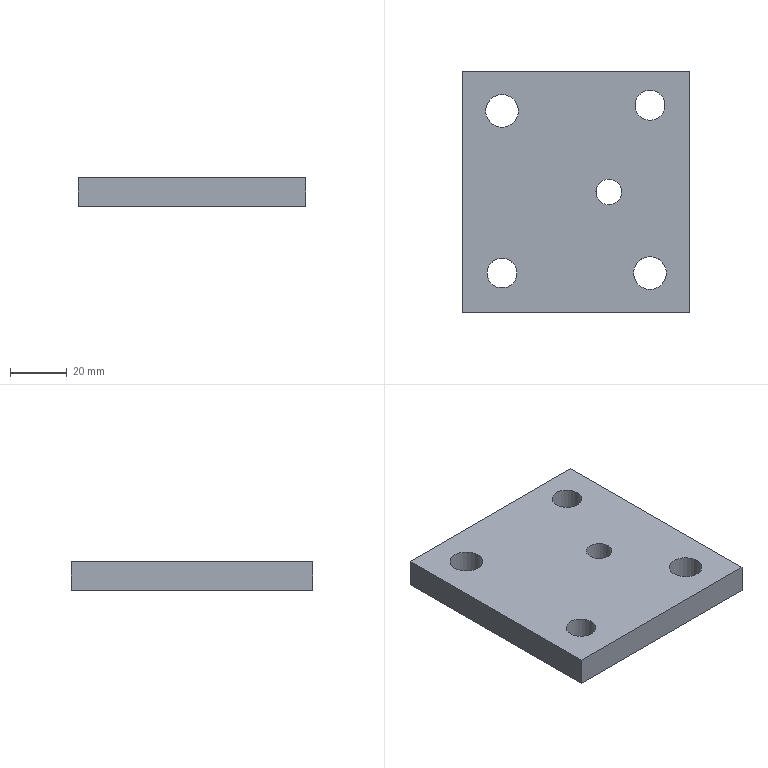Part | NX | features 6 2 | 1 solid | 11 faces | box 80 x 85 x 10 mm | volume 63555 mm3 | plane 6 | cylinder 5 | commonest cylinder face diameters 10.5 x2 11.5 x2 9 x1
STEP:
#1=CARTESIAN_POINT('',(3152.247,119.828,101.));
#2=VERTEX_POINT('',#1);
#3=CARTESIAN_POINT('',(3152.247,34.828,101.));
#4=VERTEX_POINT('',#3);
#5=CARTESIAN_POINT('',(3152.247,77.328,101.));
#6=DIRECTION('',(0.,-1.,0.));
#7=VECTOR('',#6,1000.);
#8=LINE('',#5,#7);
#9=EDGE_CURVE('',#2,#4,#8,.T.);
#10=ORIENTED_EDGE('',*,*,#9,.T.);
#11=CARTESIAN_POINT('',(3152.247,34.828,91.));
#12=VERTEX_POINT('',#11);
#13=CARTESIAN_POINT('',(3152.247,34.828,81.));
#14=DIRECTION('',(0.,0.,1.));
#15=VECTOR('',#14,1000.);
#16=LINE('',#13,#15);
#17=EDGE_CURVE('',#12,#4,#16,.T.);
#18=ORIENTED_EDGE('',*,*,#17,.F.);
#19=CARTESIAN_POINT('',(3152.247,119.828,91.));
#20=VERTEX_POINT('',#19);
#21=CARTESIAN_POINT('',(3152.247,77.328,91.));
#22=DIRECTION('',(0.,-1.,0.));
#23=VECTOR('',#22,1000.);
#24=LINE('',#21,#23);
#25=EDGE_CURVE('',#20,#12,#24,.T.);
#26=ORIENTED_EDGE('',*,*,#25,.F.);
#27=CARTESIAN_POINT('',(3152.247,119.828,81.));
#28=DIRECTION('',(0.,0.,-1.));
#29=VECTOR('',#28,1000.);
#30=LINE('',#27,#29);
#31=EDGE_CURVE('',#2,#20,#30,.T.);
#32=ORIENTED_EDGE('',*,*,#31,.F.);
#33=EDGE_LOOP('',(#10,#18,#26,#32));
#34=FACE_BOUND('',#33,.T.);
#35=CARTESIAN_POINT('',(3152.247,77.328,81.));
#36=DIRECTION('',(-1.,0.,0.));
#37=DIRECTION('',(0.,-1.,0.));
#38=AXIS2_PLACEMENT_3D('',#35,#36,#37);
#39=PLANE('',#38);
#40=ADVANCED_FACE('',(#34),#39,.F.);
#41=CARTESIAN_POINT('',(3072.247,119.828,101.));
#42=VERTEX_POINT('',#41);
#43=CARTESIAN_POINT('',(3102.247,119.828,101.));
#44=DIRECTION('',(1.,0.,0.));
#45=VECTOR('',#44,1000.);
#46=LINE('',#43,#45);
#47=EDGE_CURVE('',#42,#2,#46,.T.);
#48=ORIENTED_EDGE('',*,*,#47,.T.);
#49=ORIENTED_EDGE('',*,*,#31,.T.);
#50=CARTESIAN_POINT('',(3072.247,119.828,91.));
#51=VERTEX_POINT('',#50);
#52=CARTESIAN_POINT('',(3102.247,119.828,91.));
#53=DIRECTION('',(1.,0.,0.));
#54=VECTOR('',#53,1000.);
#55=LINE('',#52,#54);
#56=EDGE_CURVE('',#51,#20,#55,.T.);
#57=ORIENTED_EDGE('',*,*,#56,.F.);
#58=CARTESIAN_POINT('',(3072.247,119.828,81.));
#59=DIRECTION('',(0.,0.,-1.));
#60=VECTOR('',#59,1000.);
#61=LINE('',#58,#60);
#62=EDGE_CURVE('',#42,#51,#61,.T.);
#63=ORIENTED_EDGE('',*,*,#62,.F.);
#64=EDGE_LOOP('',(#48,#49,#57,#63));
#65=FACE_BOUND('',#64,.T.);
#66=CARTESIAN_POINT('',(3102.247,119.828,81.));
#67=DIRECTION('',(0.,-1.,0.));
#68=DIRECTION('',(1.,0.,0.));
#69=AXIS2_PLACEMENT_3D('',#66,#67,#68);
#70=PLANE('',#69);
#71=ADVANCED_FACE('',(#65),#70,.F.);
#72=CARTESIAN_POINT('',(3072.247,34.828,101.));
#73=VERTEX_POINT('',#72);
#74=CARTESIAN_POINT('',(3072.247,77.328,101.));
#75=DIRECTION('',(0.,1.,0.));
#76=VECTOR('',#75,1000.);
#77=LINE('',#74,#76);
#78=EDGE_CURVE('',#73,#42,#77,.T.);
#79=ORIENTED_EDGE('',*,*,#78,.T.);
#80=ORIENTED_EDGE('',*,*,#62,.T.);
#81=CARTESIAN_POINT('',(3072.247,34.828,91.));
#82=VERTEX_POINT('',#81);
#83=CARTESIAN_POINT('',(3072.247,77.328,91.));
#84=DIRECTION('',(0.,1.,0.));
#85=VECTOR('',#84,1000.);
#86=LINE('',#83,#85);
#87=EDGE_CURVE('',#82,#51,#86,.T.);
#88=ORIENTED_EDGE('',*,*,#87,.F.);
#89=CARTESIAN_POINT('',(3072.247,34.828,81.));
#90=DIRECTION('',(0.,0.,-1.));
#91=VECTOR('',#90,1000.);
#92=LINE('',#89,#91);
#93=EDGE_CURVE('',#73,#82,#92,.T.);
#94=ORIENTED_EDGE('',*,*,#93,.F.);
#95=EDGE_LOOP('',(#79,#80,#88,#94));
#96=FACE_BOUND('',#95,.T.);
#97=CARTESIAN_POINT('',(3072.247,77.328,81.));
#98=DIRECTION('',(1.,0.,0.));
#99=DIRECTION('',(0.,1.,0.));
#100=AXIS2_PLACEMENT_3D('',#97,#98,#99);
#101=PLANE('',#100);
#102=ADVANCED_FACE('',(#96),#101,.F.);
#103=CARTESIAN_POINT('',(3091.497,48.828,91.));
#104=VERTEX_POINT('',#103);
#105=CARTESIAN_POINT('',(3086.247,48.828,91.));
#106=DIRECTION('',(0.,0.,-1.));
#107=DIRECTION('',(1.,0.,0.));
#108=AXIS2_PLACEMENT_3D('',#105,#106,#107);
#109=CIRCLE('',#108,5.25);
#110=EDGE_CURVE('',#104,#104,#109,.T.);
#111=ORIENTED_EDGE('',*,*,#110,.T.);
#112=EDGE_LOOP('',(#111));
#113=FACE_BOUND('',#112,.T.);
#114=CARTESIAN_POINT('',(3080.997,48.828,101.));
#115=VERTEX_POINT('',#114);
#116=CARTESIAN_POINT('',(3086.247,48.828,101.));
#117=DIRECTION('',(0.,0.,1.));
#118=DIRECTION('',(-1.,0.,0.));
#119=AXIS2_PLACEMENT_3D('',#116,#117,#118);
#120=CIRCLE('',#119,5.25);
#121=EDGE_CURVE('',#115,#115,#120,.T.);
#122=ORIENTED_EDGE('',*,*,#121,.T.);
#123=EDGE_LOOP('',(#122));
#124=FACE_BOUND('',#123,.T.);
#125=CARTESIAN_POINT('',(3086.247,48.828,81.));
#126=DIRECTION('',(0.,0.,1.));
#127=DIRECTION('',(0.,-1.,0.));
#128=AXIS2_PLACEMENT_3D('',#125,#126,#127);
#129=CYLINDRICAL_SURFACE('',#128,5.25);
#130=ADVANCED_FACE('',(#113,#124),#129,.F.);
#131=CARTESIAN_POINT('',(3143.997,48.828,91.));
#132=VERTEX_POINT('',#131);
#133=CARTESIAN_POINT('',(3138.247,48.828,91.));
#134=DIRECTION('',(0.,0.,1.));
#135=DIRECTION('',(1.,0.,0.));
#136=AXIS2_PLACEMENT_3D('',#133,#134,#135);
#137=CIRCLE('',#136,5.75);
#138=EDGE_CURVE('',#132,#132,#137,.T.);
#139=ORIENTED_EDGE('',*,*,#138,.F.);
#140=EDGE_LOOP('',(#139));
#141=FACE_BOUND('',#140,.T.);
#142=CARTESIAN_POINT('',(3132.497,48.828,101.));
#143=VERTEX_POINT('',#142);
#144=CARTESIAN_POINT('',(3138.247,48.828,101.));
#145=DIRECTION('',(0.,0.,1.));
#146=DIRECTION('',(-1.,0.,0.));
#147=AXIS2_PLACEMENT_3D('',#144,#145,#146);
#148=CIRCLE('',#147,5.75);
#149=EDGE_CURVE('',#143,#143,#148,.T.);
#150=ORIENTED_EDGE('',*,*,#149,.T.);
#151=EDGE_LOOP('',(#150));
#152=FACE_BOUND('',#151,.T.);
#153=CARTESIAN_POINT('',(3138.247,48.828,81.));
#154=DIRECTION('',(0.,0.,1.));
#155=DIRECTION('',(0.,-1.,0.));
#156=AXIS2_PLACEMENT_3D('',#153,#154,#155);
#157=CYLINDRICAL_SURFACE('',#156,5.75);
#158=ADVANCED_FACE('',(#141,#152),#157,.F.);
#159=CARTESIAN_POINT('',(3102.247,34.828,91.));
#160=DIRECTION('',(-1.,0.,0.));
#161=VECTOR('',#160,1000.);
#162=LINE('',#159,#161);
#163=EDGE_CURVE('',#12,#82,#162,.T.);
#164=ORIENTED_EDGE('',*,*,#163,.F.);
#165=ORIENTED_EDGE('',*,*,#17,.T.);
#166=CARTESIAN_POINT('',(3102.247,34.828,101.));
#167=DIRECTION('',(-1.,0.,0.));
#168=VECTOR('',#167,1000.);
#169=LINE('',#166,#168);
#170=EDGE_CURVE('',#4,#73,#169,.T.);
#171=ORIENTED_EDGE('',*,*,#170,.T.);
#172=ORIENTED_EDGE('',*,*,#93,.T.);
#173=EDGE_LOOP('',(#164,#165,#171,#172));
#174=FACE_BOUND('',#173,.T.);
#175=CARTESIAN_POINT('',(3102.247,34.828,81.));
#176=DIRECTION('',(0.,1.,0.));
#177=DIRECTION('',(-1.,0.,0.));
#178=AXIS2_PLACEMENT_3D('',#175,#176,#177);
#179=PLANE('',#178);
#180=ADVANCED_FACE('',(#174),#179,.F.);
#181=CARTESIAN_POINT('',(3091.997,105.828,91.));
#182=VERTEX_POINT('',#181);
#183=CARTESIAN_POINT('',(3086.247,105.828,91.));
#184=DIRECTION('',(0.,0.,1.));
#185=DIRECTION('',(1.,0.,0.));
#186=AXIS2_PLACEMENT_3D('',#183,#184,#185);
#187=CIRCLE('',#186,5.75);
#188=EDGE_CURVE('',#182,#182,#187,.T.);
#189=ORIENTED_EDGE('',*,*,#188,.F.);
#190=EDGE_LOOP('',(#189));
#191=FACE_BOUND('',#190,.T.);
#192=CARTESIAN_POINT('',(3080.497,105.828,101.));
#193=VERTEX_POINT('',#192);
#194=CARTESIAN_POINT('',(3086.247,105.828,101.));
#195=DIRECTION('',(0.,0.,1.));
#196=DIRECTION('',(-1.,0.,0.));
#197=AXIS2_PLACEMENT_3D('',#194,#195,#196);
#198=CIRCLE('',#197,5.75);
#199=EDGE_CURVE('',#193,#193,#198,.T.);
#200=ORIENTED_EDGE('',*,*,#199,.T.);
#201=EDGE_LOOP('',(#200));
#202=FACE_BOUND('',#201,.T.);
#203=CARTESIAN_POINT('',(3086.247,105.828,81.));
#204=DIRECTION('',(0.,0.,1.));
#205=DIRECTION('',(0.,-1.,0.));
#206=AXIS2_PLACEMENT_3D('',#203,#204,#205);
#207=CYLINDRICAL_SURFACE('',#206,5.75);
#208=ADVANCED_FACE('',(#191,#202),#207,.F.);
#209=CARTESIAN_POINT('',(3143.497,107.828,91.));
#210=VERTEX_POINT('',#209);
#211=CARTESIAN_POINT('',(3138.247,107.828,91.));
#212=DIRECTION('',(0.,0.,-1.));
#213=DIRECTION('',(1.,0.,0.));
#214=AXIS2_PLACEMENT_3D('',#211,#212,#213);
#215=CIRCLE('',#214,5.25);
#216=EDGE_CURVE('',#210,#210,#215,.T.);
#217=ORIENTED_EDGE('',*,*,#216,.T.);
#218=EDGE_LOOP('',(#217));
#219=FACE_BOUND('',#218,.T.);
#220=CARTESIAN_POINT('',(3132.997,107.828,101.));
#221=VERTEX_POINT('',#220);
#222=CARTESIAN_POINT('',(3138.247,107.828,101.));
#223=DIRECTION('',(0.,0.,1.));
#224=DIRECTION('',(-1.,0.,0.));
#225=AXIS2_PLACEMENT_3D('',#222,#223,#224);
#226=CIRCLE('',#225,5.25);
#227=EDGE_CURVE('',#221,#221,#226,.T.);
#228=ORIENTED_EDGE('',*,*,#227,.T.);
#229=EDGE_LOOP('',(#228));
#230=FACE_BOUND('',#229,.T.);
#231=CARTESIAN_POINT('',(3138.247,107.828,81.));
#232=DIRECTION('',(0.,0.,1.));
#233=DIRECTION('',(0.,-1.,0.));
#234=AXIS2_PLACEMENT_3D('',#231,#232,#233);
#235=CYLINDRICAL_SURFACE('',#234,5.25);
#236=ADVANCED_FACE('',(#219,#230),#235,.F.);
#237=CARTESIAN_POINT('',(3128.247,77.328,91.));
#238=VERTEX_POINT('',#237);
#239=CARTESIAN_POINT('',(3123.747,77.328,91.));
#240=DIRECTION('',(0.,0.,-1.));
#241=DIRECTION('',(1.,0.,0.));
#242=AXIS2_PLACEMENT_3D('',#239,#240,#241);
#243=CIRCLE('',#242,4.5);
#244=EDGE_CURVE('',#238,#238,#243,.T.);
#245=ORIENTED_EDGE('',*,*,#244,.T.);
#246=EDGE_LOOP('',(#245));
#247=FACE_BOUND('',#246,.T.);
#248=CARTESIAN_POINT('',(3119.247,77.328,101.));
#249=VERTEX_POINT('',#248);
#250=CARTESIAN_POINT('',(3123.747,77.328,101.));
#251=DIRECTION('',(0.,0.,1.));
#252=DIRECTION('',(-1.,0.,0.));
#253=AXIS2_PLACEMENT_3D('',#250,#251,#252);
#254=CIRCLE('',#253,4.5);
#255=EDGE_CURVE('',#249,#249,#254,.T.);
#256=ORIENTED_EDGE('',*,*,#255,.T.);
#257=EDGE_LOOP('',(#256));
#258=FACE_BOUND('',#257,.T.);
#259=CARTESIAN_POINT('',(3123.747,77.328,-129.));
#260=DIRECTION('',(0.,0.,1.));
#261=DIRECTION('',(0.,-1.,0.));
#262=AXIS2_PLACEMENT_3D('',#259,#260,#261);
#263=CYLINDRICAL_SURFACE('',#262,4.5);
#264=ADVANCED_FACE('',(#247,#258),#263,.F.);
#265=ORIENTED_EDGE('',*,*,#216,.F.);
#266=EDGE_LOOP('',(#265));
#267=FACE_BOUND('',#266,.T.);
#268=ORIENTED_EDGE('',*,*,#188,.T.);
#269=EDGE_LOOP('',(#268));
#270=FACE_BOUND('',#269,.T.);
#271=ORIENTED_EDGE('',*,*,#87,.T.);
#272=ORIENTED_EDGE('',*,*,#56,.T.);
#273=ORIENTED_EDGE('',*,*,#25,.T.);
#274=ORIENTED_EDGE('',*,*,#163,.T.);
#275=EDGE_LOOP('',(#271,#272,#273,#274));
#276=FACE_BOUND('',#275,.T.);
#277=ORIENTED_EDGE('',*,*,#138,.T.);
#278=EDGE_LOOP('',(#277));
#279=FACE_BOUND('',#278,.T.);
#280=ORIENTED_EDGE('',*,*,#110,.F.);
#281=EDGE_LOOP('',(#280));
#282=FACE_BOUND('',#281,.T.);
#283=ORIENTED_EDGE('',*,*,#244,.F.);
#284=EDGE_LOOP('',(#283));
#285=FACE_BOUND('',#284,.T.);
#286=CARTESIAN_POINT('',(3102.247,77.328,91.));
#287=DIRECTION('',(0.,0.,1.));
#288=DIRECTION('',(0.,-1.,0.));
#289=AXIS2_PLACEMENT_3D('',#286,#287,#288);
#290=PLANE('',#289);
#291=ADVANCED_FACE('',(#267,#270,#276,#279,#282,#285),#290,.F.);
#292=ORIENTED_EDGE('',*,*,#121,.F.);
#293=EDGE_LOOP('',(#292));
#294=FACE_BOUND('',#293,.T.);
#295=ORIENTED_EDGE('',*,*,#149,.F.);
#296=EDGE_LOOP('',(#295));
#297=FACE_BOUND('',#296,.T.);
#298=ORIENTED_EDGE('',*,*,#170,.F.);
#299=ORIENTED_EDGE('',*,*,#9,.F.);
#300=ORIENTED_EDGE('',*,*,#47,.F.);
#301=ORIENTED_EDGE('',*,*,#78,.F.);
#302=EDGE_LOOP('',(#298,#299,#300,#301));
#303=FACE_BOUND('',#302,.T.);
#304=ORIENTED_EDGE('',*,*,#199,.F.);
#305=EDGE_LOOP('',(#304));
#306=FACE_BOUND('',#305,.T.);
#307=ORIENTED_EDGE('',*,*,#227,.F.);
#308=EDGE_LOOP('',(#307));
#309=FACE_BOUND('',#308,.T.);
#310=ORIENTED_EDGE('',*,*,#255,.F.);
#311=EDGE_LOOP('',(#310));
#312=FACE_BOUND('',#311,.T.);
#313=CARTESIAN_POINT('',(3200.056,1242.718,101.));
#314=DIRECTION('',(0.,0.,1.));
#315=DIRECTION('',(0.,1.,0.));
#316=AXIS2_PLACEMENT_3D('',#313,#314,#315);
#317=PLANE('',#316);
#318=ADVANCED_FACE('',(#294,#297,#303,#306,#309,#312),#317,.T.);
#319=CLOSED_SHELL('',(#40,#71,#102,#130,#158,#180,#208,#236,#264,#291,#318));
#320=MANIFOLD_SOLID_BREP('',#319);
#321=(LENGTH_UNIT()NAMED_UNIT(*)SI_UNIT(.MILLI.,.METRE.));
#322=UNCERTAINTY_MEASURE_WITH_UNIT(LENGTH_MEASURE(0.00001),#321,'','');
#323=(NAMED_UNIT(*)PLANE_ANGLE_UNIT()SI_UNIT($,.RADIAN.));
#324=(NAMED_UNIT(*)SI_UNIT($,.STERADIAN.)SOLID_ANGLE_UNIT());
#325=(GEOMETRIC_REPRESENTATION_CONTEXT(3)GLOBAL_UNCERTAINTY_ASSIGNED_CONTEXT((#322))GLOBAL_UNIT_ASSIGNED_CONTEXT((#321,#323,#324))REPRESENTATION_CONTEXT('',''));
#326=ADVANCED_BREP_SHAPE_REPRESENTATION('',(#320),#325);